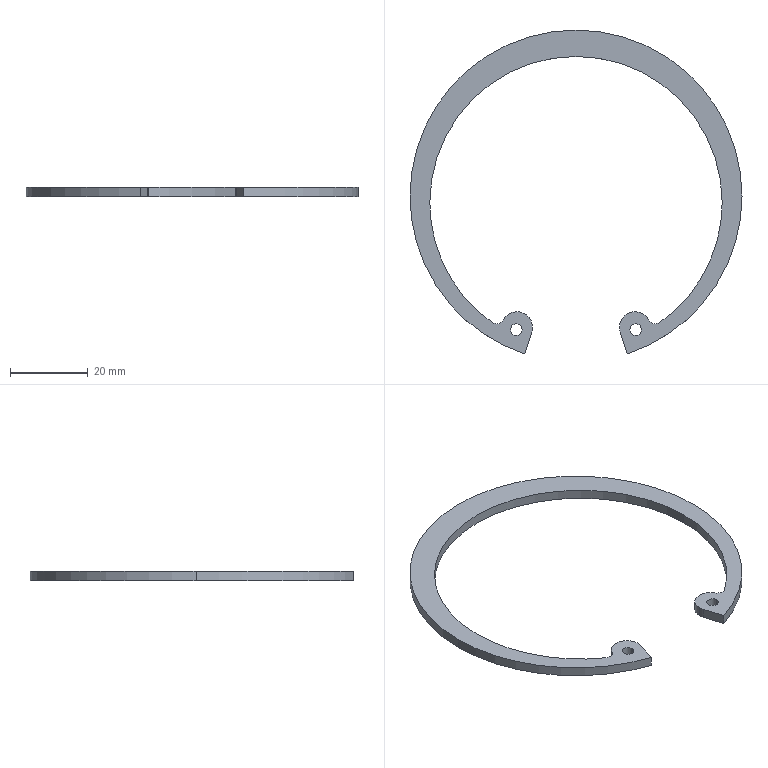Part | SolidWorks | features Extrusion 1 | 1 solid | 19 faces | box 85.5 x 83.408 x 2.5 mm | volume 3180 mm3 | cylinder 15 | plane 4 | commonest cylinder face diameters 3 x4 8 x3 75.3 x3 85.5 x3 4 x2
STEP:
#1=CARTESIAN_POINT('',(13.888,-34.416,1.25));
#2=VERTEX_POINT('',#1);
#3=CARTESIAN_POINT('',(16.888,-34.416,1.25));
#4=VERTEX_POINT('',#3);
#5=CARTESIAN_POINT('',(15.388,-34.416,1.25));
#6=DIRECTION('',(0.,0.,1.));
#7=DIRECTION('',(-1.,0.,0.));
#8=AXIS2_PLACEMENT_3D('',#5,#6,#7);
#9=CIRCLE('',#8,1.5);
#10=EDGE_CURVE('',#2,#4,#9,.T.);
#11=ORIENTED_EDGE('',*,*,#10,.T.);
#12=CARTESIAN_POINT('',(16.888,-34.416,-1.25));
#13=VERTEX_POINT('',#12);
#14=CARTESIAN_POINT('',(16.888,-34.416,1.25));
#15=DIRECTION('',(0.,0.,-1.));
#16=VECTOR('',#15,1000.);
#17=LINE('',#14,#16);
#18=EDGE_CURVE('',#4,#13,#17,.T.);
#19=ORIENTED_EDGE('',*,*,#18,.T.);
#20=CARTESIAN_POINT('',(13.888,-34.416,-1.25));
#21=VERTEX_POINT('',#20);
#22=CARTESIAN_POINT('',(15.388,-34.416,-1.25));
#23=DIRECTION('',(0.,0.,1.));
#24=DIRECTION('',(-1.,0.,0.));
#25=AXIS2_PLACEMENT_3D('',#22,#23,#24);
#26=CIRCLE('',#25,1.5);
#27=EDGE_CURVE('',#21,#13,#26,.T.);
#28=ORIENTED_EDGE('',*,*,#27,.F.);
#29=CARTESIAN_POINT('',(13.888,-34.416,1.25));
#30=DIRECTION('',(0.,0.,-1.));
#31=VECTOR('',#30,1000.);
#32=LINE('',#29,#31);
#33=EDGE_CURVE('',#2,#21,#32,.T.);
#34=ORIENTED_EDGE('',*,*,#33,.F.);
#35=EDGE_LOOP('',(#11,#19,#28,#34));
#36=FACE_OUTER_BOUND('',#35,.T.);
#37=CARTESIAN_POINT('',(15.388,-34.416,1.25));
#38=DIRECTION('',(0.,0.,-1.));
#39=DIRECTION('',(-1.,0.,0.));
#40=AXIS2_PLACEMENT_3D('',#37,#38,#39);
#41=CYLINDRICAL_SURFACE('',#40,1.5);
#42=ADVANCED_FACE('',(#36),#41,.F.);
#43=CARTESIAN_POINT('',(-16.888,-34.416,1.25));
#44=VERTEX_POINT('',#43);
#45=CARTESIAN_POINT('',(-13.888,-34.416,1.25));
#46=VERTEX_POINT('',#45);
#47=CARTESIAN_POINT('',(-15.388,-34.416,1.25));
#48=DIRECTION('',(0.,0.,1.));
#49=DIRECTION('',(1.,0.,0.));
#50=AXIS2_PLACEMENT_3D('',#47,#48,#49);
#51=CIRCLE('',#50,1.5);
#52=EDGE_CURVE('',#44,#46,#51,.T.);
#53=ORIENTED_EDGE('',*,*,#52,.T.);
#54=CARTESIAN_POINT('',(-13.888,-34.416,-1.25));
#55=VERTEX_POINT('',#54);
#56=CARTESIAN_POINT('',(-13.888,-34.416,1.25));
#57=DIRECTION('',(0.,0.,-1.));
#58=VECTOR('',#57,1000.);
#59=LINE('',#56,#58);
#60=EDGE_CURVE('',#46,#55,#59,.T.);
#61=ORIENTED_EDGE('',*,*,#60,.T.);
#62=CARTESIAN_POINT('',(-16.888,-34.416,-1.25));
#63=VERTEX_POINT('',#62);
#64=CARTESIAN_POINT('',(-15.388,-34.416,-1.25));
#65=DIRECTION('',(0.,0.,1.));
#66=DIRECTION('',(1.,0.,0.));
#67=AXIS2_PLACEMENT_3D('',#64,#65,#66);
#68=CIRCLE('',#67,1.5);
#69=EDGE_CURVE('',#63,#55,#68,.T.);
#70=ORIENTED_EDGE('',*,*,#69,.F.);
#71=CARTESIAN_POINT('',(-16.888,-34.416,1.25));
#72=DIRECTION('',(0.,0.,-1.));
#73=VECTOR('',#72,1000.);
#74=LINE('',#71,#73);
#75=EDGE_CURVE('',#44,#63,#74,.T.);
#76=ORIENTED_EDGE('',*,*,#75,.F.);
#77=EDGE_LOOP('',(#53,#61,#70,#76));
#78=FACE_OUTER_BOUND('',#77,.T.);
#79=CARTESIAN_POINT('',(-15.388,-34.416,1.25));
#80=DIRECTION('',(0.,0.,-1.));
#81=DIRECTION('',(-1.,0.,0.));
#82=AXIS2_PLACEMENT_3D('',#79,#80,#81);
#83=CYLINDRICAL_SURFACE('',#82,1.5);
#84=ADVANCED_FACE('',(#78),#83,.F.);
#85=CARTESIAN_POINT('',(42.75,0.,1.25));
#86=VERTEX_POINT('',#85);
#87=CARTESIAN_POINT('',(-42.75,0.,1.25));
#88=VERTEX_POINT('',#87);
#89=CARTESIAN_POINT('',(0.,0.,1.25));
#90=DIRECTION('',(0.,0.,1.));
#91=DIRECTION('',(1.,0.,0.));
#92=AXIS2_PLACEMENT_3D('',#89,#90,#91);
#93=CIRCLE('',#92,42.75);
#94=EDGE_CURVE('',#86,#88,#93,.T.);
#95=ORIENTED_EDGE('',*,*,#94,.F.);
#96=CARTESIAN_POINT('',(42.75,0.,-1.25));
#97=VERTEX_POINT('',#96);
#98=CARTESIAN_POINT('',(42.75,0.,1.25));
#99=DIRECTION('',(0.,0.,-1.));
#100=VECTOR('',#99,1000.);
#101=LINE('',#98,#100);
#102=EDGE_CURVE('',#86,#97,#101,.T.);
#103=ORIENTED_EDGE('',*,*,#102,.T.);
#104=CARTESIAN_POINT('',(-42.75,0.,-1.25));
#105=VERTEX_POINT('',#104);
#106=CARTESIAN_POINT('',(0.,0.,-1.25));
#107=DIRECTION('',(0.,0.,1.));
#108=DIRECTION('',(1.,0.,0.));
#109=AXIS2_PLACEMENT_3D('',#106,#107,#108);
#110=CIRCLE('',#109,42.75);
#111=EDGE_CURVE('',#97,#105,#110,.T.);
#112=ORIENTED_EDGE('',*,*,#111,.T.);
#113=CARTESIAN_POINT('',(-42.75,0.,1.25));
#114=DIRECTION('',(0.,0.,-1.));
#115=VECTOR('',#114,1000.);
#116=LINE('',#113,#115);
#117=EDGE_CURVE('',#88,#105,#116,.T.);
#118=ORIENTED_EDGE('',*,*,#117,.F.);
#119=EDGE_LOOP('',(#95,#103,#112,#118));
#120=FACE_OUTER_BOUND('',#119,.T.);
#121=CARTESIAN_POINT('',(0.,0.,1.25));
#122=DIRECTION('',(0.,0.,-1.));
#123=DIRECTION('',(-1.,0.,0.));
#124=AXIS2_PLACEMENT_3D('',#121,#122,#123);
#125=CYLINDRICAL_SURFACE('',#124,42.75);
#126=ADVANCED_FACE('',(#120),#125,.T.);
#127=CARTESIAN_POINT('',(-13.21,-40.658,1.25));
#128=VERTEX_POINT('',#127);
#129=CARTESIAN_POINT('',(0.,0.,1.25));
#130=DIRECTION('',(0.,0.,1.));
#131=DIRECTION('',(1.,0.,0.));
#132=AXIS2_PLACEMENT_3D('',#129,#130,#131);
#133=CIRCLE('',#132,42.75);
#134=EDGE_CURVE('',#88,#128,#133,.T.);
#135=ORIENTED_EDGE('',*,*,#134,.F.);
#136=ORIENTED_EDGE('',*,*,#117,.T.);
#137=CARTESIAN_POINT('',(-13.21,-40.658,-1.25));
#138=VERTEX_POINT('',#137);
#139=CARTESIAN_POINT('',(0.,0.,-1.25));
#140=DIRECTION('',(0.,0.,1.));
#141=DIRECTION('',(1.,0.,0.));
#142=AXIS2_PLACEMENT_3D('',#139,#140,#141);
#143=CIRCLE('',#142,42.75);
#144=EDGE_CURVE('',#105,#138,#143,.T.);
#145=ORIENTED_EDGE('',*,*,#144,.T.);
#146=CARTESIAN_POINT('',(-13.21,-40.658,1.25));
#147=DIRECTION('',(0.,0.,-1.));
#148=VECTOR('',#147,1000.);
#149=LINE('',#146,#148);
#150=EDGE_CURVE('',#128,#138,#149,.T.);
#151=ORIENTED_EDGE('',*,*,#150,.F.);
#152=EDGE_LOOP('',(#135,#136,#145,#151));
#153=FACE_OUTER_BOUND('',#152,.T.);
#154=CARTESIAN_POINT('',(0.,0.,1.25));
#155=DIRECTION('',(0.,0.,-1.));
#156=DIRECTION('',(-1.,0.,0.));
#157=AXIS2_PLACEMENT_3D('',#154,#155,#156);
#158=CYLINDRICAL_SURFACE('',#157,42.75);
#159=ADVANCED_FACE('',(#153),#158,.T.);
#160=CARTESIAN_POINT('',(11.186,-33.795,1.25));
#161=VERTEX_POINT('',#160);
#162=CARTESIAN_POINT('',(11.382,-35.031,1.25));
#163=VERTEX_POINT('',#162);
#164=CARTESIAN_POINT('',(15.186,-33.795,1.25));
#165=DIRECTION('',(0.,0.,1.));
#166=DIRECTION('',(-1.,0.,0.));
#167=AXIS2_PLACEMENT_3D('',#164,#165,#166);
#168=CIRCLE('',#167,4.);
#169=EDGE_CURVE('',#161,#163,#168,.T.);
#170=ORIENTED_EDGE('',*,*,#169,.F.);
#171=CARTESIAN_POINT('',(11.186,-33.795,-1.25));
#172=VERTEX_POINT('',#171);
#173=CARTESIAN_POINT('',(11.186,-33.795,1.25));
#174=DIRECTION('',(0.,0.,-1.));
#175=VECTOR('',#174,1000.);
#176=LINE('',#173,#175);
#177=EDGE_CURVE('',#161,#172,#176,.T.);
#178=ORIENTED_EDGE('',*,*,#177,.T.);
#179=CARTESIAN_POINT('',(11.382,-35.031,-1.25));
#180=VERTEX_POINT('',#179);
#181=CARTESIAN_POINT('',(15.186,-33.795,-1.25));
#182=DIRECTION('',(0.,0.,1.));
#183=DIRECTION('',(-1.,0.,0.));
#184=AXIS2_PLACEMENT_3D('',#181,#182,#183);
#185=CIRCLE('',#184,4.);
#186=EDGE_CURVE('',#172,#180,#185,.T.);
#187=ORIENTED_EDGE('',*,*,#186,.T.);
#188=CARTESIAN_POINT('',(11.382,-35.031,1.25));
#189=DIRECTION('',(0.,0.,-1.));
#190=VECTOR('',#189,1000.);
#191=LINE('',#188,#190);
#192=EDGE_CURVE('',#163,#180,#191,.T.);
#193=ORIENTED_EDGE('',*,*,#192,.F.);
#194=EDGE_LOOP('',(#170,#178,#187,#193));
#195=FACE_OUTER_BOUND('',#194,.T.);
#196=CARTESIAN_POINT('',(15.186,-33.795,1.25));
#197=DIRECTION('',(0.,0.,-1.));
#198=DIRECTION('',(-1.,0.,0.));
#199=AXIS2_PLACEMENT_3D('',#196,#197,#198);
#200=CYLINDRICAL_SURFACE('',#199,4.);
#201=ADVANCED_FACE('',(#195),#200,.T.);
#202=CARTESIAN_POINT('',(37.65,-1.7,1.25));
#203=VERTEX_POINT('',#202);
#204=CARTESIAN_POINT('',(21.592,-32.543,1.25));
#205=VERTEX_POINT('',#204);
#206=CARTESIAN_POINT('',(0.,-1.7,1.25));
#207=DIRECTION('',(0.,0.,-1.));
#208=DIRECTION('',(1.,0.,0.));
#209=AXIS2_PLACEMENT_3D('',#206,#207,#208);
#210=CIRCLE('',#209,37.65);
#211=EDGE_CURVE('',#203,#205,#210,.T.);
#212=ORIENTED_EDGE('',*,*,#211,.F.);
#213=CARTESIAN_POINT('',(37.65,-1.7,-1.25));
#214=VERTEX_POINT('',#213);
#215=CARTESIAN_POINT('',(37.65,-1.7,1.25));
#216=DIRECTION('',(0.,0.,-1.));
#217=VECTOR('',#216,1000.);
#218=LINE('',#215,#217);
#219=EDGE_CURVE('',#203,#214,#218,.T.);
#220=ORIENTED_EDGE('',*,*,#219,.T.);
#221=CARTESIAN_POINT('',(21.592,-32.543,-1.25));
#222=VERTEX_POINT('',#221);
#223=CARTESIAN_POINT('',(0.,-1.7,-1.25));
#224=DIRECTION('',(0.,0.,-1.));
#225=DIRECTION('',(1.,0.,0.));
#226=AXIS2_PLACEMENT_3D('',#223,#224,#225);
#227=CIRCLE('',#226,37.65);
#228=EDGE_CURVE('',#214,#222,#227,.T.);
#229=ORIENTED_EDGE('',*,*,#228,.T.);
#230=CARTESIAN_POINT('',(21.592,-32.543,1.25));
#231=DIRECTION('',(0.,0.,-1.));
#232=VECTOR('',#231,1000.);
#233=LINE('',#230,#232);
#234=EDGE_CURVE('',#205,#222,#233,.T.);
#235=ORIENTED_EDGE('',*,*,#234,.F.);
#236=EDGE_LOOP('',(#212,#220,#229,#235));
#237=FACE_OUTER_BOUND('',#236,.T.);
#238=CARTESIAN_POINT('',(0.,-1.7,1.25));
#239=DIRECTION('',(0.,0.,-1.));
#240=DIRECTION('',(-1.,0.,0.));
#241=AXIS2_PLACEMENT_3D('',#238,#239,#240);
#242=CYLINDRICAL_SURFACE('',#241,37.65);
#243=ADVANCED_FACE('',(#237),#242,.F.);
#244=ORIENTED_EDGE('',*,*,#219,.F.);
#245=CARTESIAN_POINT('',(-37.65,-1.7,1.25));
#246=VERTEX_POINT('',#245);
#247=CARTESIAN_POINT('',(0.,-1.7,1.25));
#248=DIRECTION('',(0.,0.,-1.));
#249=DIRECTION('',(1.,0.,0.));
#250=AXIS2_PLACEMENT_3D('',#247,#248,#249);
#251=CIRCLE('',#250,37.65);
#252=EDGE_CURVE('',#246,#203,#251,.T.);
#253=ORIENTED_EDGE('',*,*,#252,.F.);
#254=CARTESIAN_POINT('',(-37.65,-1.7,-1.25));
#255=VERTEX_POINT('',#254);
#256=CARTESIAN_POINT('',(-37.65,-1.7,1.25));
#257=DIRECTION('',(0.,0.,-1.));
#258=VECTOR('',#257,1000.);
#259=LINE('',#256,#258);
#260=EDGE_CURVE('',#246,#255,#259,.T.);
#261=ORIENTED_EDGE('',*,*,#260,.T.);
#262=CARTESIAN_POINT('',(0.,-1.7,-1.25));
#263=DIRECTION('',(0.,0.,-1.));
#264=DIRECTION('',(1.,0.,0.));
#265=AXIS2_PLACEMENT_3D('',#262,#263,#264);
#266=CIRCLE('',#265,37.65);
#267=EDGE_CURVE('',#255,#214,#266,.T.);
#268=ORIENTED_EDGE('',*,*,#267,.T.);
#269=EDGE_LOOP('',(#244,#253,#261,#268));
#270=FACE_OUTER_BOUND('',#269,.T.);
#271=CARTESIAN_POINT('',(0.,-1.7,1.25));
#272=DIRECTION('',(0.,0.,-1.));
#273=DIRECTION('',(-1.,0.,0.));
#274=AXIS2_PLACEMENT_3D('',#271,#272,#273);
#275=CYLINDRICAL_SURFACE('',#274,37.65);
#276=ADVANCED_FACE('',(#270),#275,.F.);
#277=ORIENTED_EDGE('',*,*,#52,.F.);
#278=CARTESIAN_POINT('',(-15.388,-34.416,1.25));
#279=DIRECTION('',(0.,0.,1.));
#280=DIRECTION('',(1.,0.,0.));
#281=AXIS2_PLACEMENT_3D('',#278,#279,#280);
#282=CIRCLE('',#281,1.5);
#283=EDGE_CURVE('',#46,#44,#282,.T.);
#284=ORIENTED_EDGE('',*,*,#283,.F.);
#285=EDGE_LOOP('',(#277,#284));
#286=FACE_BOUND('',#285,.T.);
#287=CARTESIAN_POINT('',(-11.382,-35.031,1.25));
#288=VERTEX_POINT('',#287);
#289=CARTESIAN_POINT('',(-18.692,-31.868,1.25));
#290=VERTEX_POINT('',#289);
#291=CARTESIAN_POINT('',(-15.186,-33.795,1.25));
#292=DIRECTION('',(0.,0.,1.));
#293=DIRECTION('',(1.,0.,0.));
#294=AXIS2_PLACEMENT_3D('',#291,#292,#293);
#295=CIRCLE('',#294,4.);
#296=EDGE_CURVE('',#288,#290,#295,.T.);
#297=ORIENTED_EDGE('',*,*,#296,.T.);
#298=CARTESIAN_POINT('',(-21.592,-32.543,1.25));
#299=VERTEX_POINT('',#298);
#300=CARTESIAN_POINT('',(-20.445,-30.905,1.25));
#301=DIRECTION('',(0.,0.,-1.));
#302=DIRECTION('',(-1.,0.,0.));
#303=AXIS2_PLACEMENT_3D('',#300,#301,#302);
#304=CIRCLE('',#303,2.);
#305=EDGE_CURVE('',#290,#299,#304,.T.);
#306=ORIENTED_EDGE('',*,*,#305,.T.);
#307=CARTESIAN_POINT('',(0.,-1.7,1.25));
#308=DIRECTION('',(0.,0.,-1.));
#309=DIRECTION('',(1.,0.,0.));
#310=AXIS2_PLACEMENT_3D('',#307,#308,#309);
#311=CIRCLE('',#310,37.65);
#312=EDGE_CURVE('',#299,#246,#311,.T.);
#313=ORIENTED_EDGE('',*,*,#312,.T.);
#314=ORIENTED_EDGE('',*,*,#252,.T.);
#315=ORIENTED_EDGE('',*,*,#211,.T.);
#316=CARTESIAN_POINT('',(18.692,-31.868,1.25));
#317=VERTEX_POINT('',#316);
#318=CARTESIAN_POINT('',(20.445,-30.905,1.25));
#319=DIRECTION('',(0.,0.,-1.));
#320=DIRECTION('',(1.,0.,0.));
#321=AXIS2_PLACEMENT_3D('',#318,#319,#320);
#322=CIRCLE('',#321,2.);
#323=EDGE_CURVE('',#205,#317,#322,.T.);
#324=ORIENTED_EDGE('',*,*,#323,.T.);
#325=CARTESIAN_POINT('',(15.186,-33.795,1.25));
#326=DIRECTION('',(0.,0.,1.));
#327=DIRECTION('',(-1.,0.,0.));
#328=AXIS2_PLACEMENT_3D('',#325,#326,#327);
#329=CIRCLE('',#328,4.);
#330=EDGE_CURVE('',#317,#161,#329,.T.);
#331=ORIENTED_EDGE('',*,*,#330,.T.);
#332=ORIENTED_EDGE('',*,*,#169,.T.);
#333=CARTESIAN_POINT('',(13.21,-40.658,1.25));
#334=VERTEX_POINT('',#333);
#335=CARTESIAN_POINT('',(11.382,-35.031,1.25));
#336=DIRECTION('',(0.309,-0.9511,0.));
#337=VECTOR('',#336,1000.);
#338=LINE('',#335,#337);
#339=EDGE_CURVE('',#163,#334,#338,.T.);
#340=ORIENTED_EDGE('',*,*,#339,.T.);
#341=CARTESIAN_POINT('',(0.,0.,1.25));
#342=DIRECTION('',(0.,0.,1.));
#343=DIRECTION('',(1.,0.,0.));
#344=AXIS2_PLACEMENT_3D('',#341,#342,#343);
#345=CIRCLE('',#344,42.75);
#346=EDGE_CURVE('',#334,#86,#345,.T.);
#347=ORIENTED_EDGE('',*,*,#346,.T.);
#348=ORIENTED_EDGE('',*,*,#94,.T.);
#349=ORIENTED_EDGE('',*,*,#134,.T.);
#350=CARTESIAN_POINT('',(-11.382,-35.031,1.25));
#351=DIRECTION('',(0.309,0.9511,0.));
#352=VECTOR('',#351,1000.);
#353=LINE('',#350,#352);
#354=EDGE_CURVE('',#128,#288,#353,.T.);
#355=ORIENTED_EDGE('',*,*,#354,.T.);
#356=EDGE_LOOP('',(#297,#306,#313,#314,#315,#324,#331,#332,#340,#347,#348,#349,#355));
#357=FACE_OUTER_BOUND('',#356,.T.);
#358=ORIENTED_EDGE('',*,*,#10,.F.);
#359=CARTESIAN_POINT('',(15.388,-34.416,1.25));
#360=DIRECTION('',(0.,0.,1.));
#361=DIRECTION('',(-1.,0.,0.));
#362=AXIS2_PLACEMENT_3D('',#359,#360,#361);
#363=CIRCLE('',#362,1.5);
#364=EDGE_CURVE('',#4,#2,#363,.T.);
#365=ORIENTED_EDGE('',*,*,#364,.F.);
#366=EDGE_LOOP('',(#358,#365));
#367=FACE_BOUND('',#366,.T.);
#368=CARTESIAN_POINT('',(-15.186,-33.795,1.25));
#369=DIRECTION('',(0.,0.,1.));
#370=DIRECTION('',(1.,0.,0.));
#371=AXIS2_PLACEMENT_3D('',#368,#369,#370);
#372=PLANE('',#371);
#373=ADVANCED_FACE('',(#286,#357,#367),#372,.T.);
#374=CARTESIAN_POINT('',(-11.382,-35.031,-1.25));
#375=VERTEX_POINT('',#374);
#376=CARTESIAN_POINT('',(-11.382,-35.031,1.25));
#377=DIRECTION('',(0.,0.,-1.));
#378=VECTOR('',#377,1000.);
#379=LINE('',#376,#378);
#380=EDGE_CURVE('',#288,#375,#379,.T.);
#381=ORIENTED_EDGE('',*,*,#380,.T.);
#382=CARTESIAN_POINT('',(-18.692,-31.868,-1.25));
#383=VERTEX_POINT('',#382);
#384=CARTESIAN_POINT('',(-15.186,-33.795,-1.25));
#385=DIRECTION('',(0.,0.,1.));
#386=DIRECTION('',(1.,0.,0.));
#387=AXIS2_PLACEMENT_3D('',#384,#385,#386);
#388=CIRCLE('',#387,4.);
#389=EDGE_CURVE('',#375,#383,#388,.T.);
#390=ORIENTED_EDGE('',*,*,#389,.T.);
#391=CARTESIAN_POINT('',(-18.692,-31.868,1.25));
#392=DIRECTION('',(0.,0.,-1.));
#393=VECTOR('',#392,1000.);
#394=LINE('',#391,#393);
#395=EDGE_CURVE('',#290,#383,#394,.T.);
#396=ORIENTED_EDGE('',*,*,#395,.F.);
#397=ORIENTED_EDGE('',*,*,#296,.F.);
#398=EDGE_LOOP('',(#381,#390,#396,#397));
#399=FACE_OUTER_BOUND('',#398,.T.);
#400=CARTESIAN_POINT('',(-15.186,-33.795,1.25));
#401=DIRECTION('',(0.,0.,-1.));
#402=DIRECTION('',(-1.,0.,0.));
#403=AXIS2_PLACEMENT_3D('',#400,#401,#402);
#404=CYLINDRICAL_SURFACE('',#403,4.);
#405=ADVANCED_FACE('',(#399),#404,.T.);
#406=ORIENTED_EDGE('',*,*,#395,.T.);
#407=CARTESIAN_POINT('',(-21.592,-32.543,-1.25));
#408=VERTEX_POINT('',#407);
#409=CARTESIAN_POINT('',(-20.445,-30.905,-1.25));
#410=DIRECTION('',(0.,0.,-1.));
#411=DIRECTION('',(-1.,0.,0.));
#412=AXIS2_PLACEMENT_3D('',#409,#410,#411);
#413=CIRCLE('',#412,2.);
#414=EDGE_CURVE('',#383,#408,#413,.T.);
#415=ORIENTED_EDGE('',*,*,#414,.T.);
#416=CARTESIAN_POINT('',(-21.592,-32.543,1.25));
#417=DIRECTION('',(0.,0.,-1.));
#418=VECTOR('',#417,1000.);
#419=LINE('',#416,#418);
#420=EDGE_CURVE('',#299,#408,#419,.T.);
#421=ORIENTED_EDGE('',*,*,#420,.F.);
#422=ORIENTED_EDGE('',*,*,#305,.F.);
#423=EDGE_LOOP('',(#406,#415,#421,#422));
#424=FACE_OUTER_BOUND('',#423,.T.);
#425=CARTESIAN_POINT('',(-20.445,-30.905,1.25));
#426=DIRECTION('',(0.,0.,-1.));
#427=DIRECTION('',(-1.,0.,0.));
#428=AXIS2_PLACEMENT_3D('',#425,#426,#427);
#429=CYLINDRICAL_SURFACE('',#428,2.);
#430=ADVANCED_FACE('',(#424),#429,.F.);
#431=ORIENTED_EDGE('',*,*,#260,.F.);
#432=ORIENTED_EDGE('',*,*,#312,.F.);
#433=ORIENTED_EDGE('',*,*,#420,.T.);
#434=CARTESIAN_POINT('',(0.,-1.7,-1.25));
#435=DIRECTION('',(0.,0.,-1.));
#436=DIRECTION('',(1.,0.,0.));
#437=AXIS2_PLACEMENT_3D('',#434,#435,#436);
#438=CIRCLE('',#437,37.65);
#439=EDGE_CURVE('',#408,#255,#438,.T.);
#440=ORIENTED_EDGE('',*,*,#439,.T.);
#441=EDGE_LOOP('',(#431,#432,#433,#440));
#442=FACE_OUTER_BOUND('',#441,.T.);
#443=CARTESIAN_POINT('',(0.,-1.7,1.25));
#444=DIRECTION('',(0.,0.,-1.));
#445=DIRECTION('',(-1.,0.,0.));
#446=AXIS2_PLACEMENT_3D('',#443,#444,#445);
#447=CYLINDRICAL_SURFACE('',#446,37.65);
#448=ADVANCED_FACE('',(#442),#447,.F.);
#449=ORIENTED_EDGE('',*,*,#234,.T.);
#450=CARTESIAN_POINT('',(18.692,-31.868,-1.25));
#451=VERTEX_POINT('',#450);
#452=CARTESIAN_POINT('',(20.445,-30.905,-1.25));
#453=DIRECTION('',(0.,0.,-1.));
#454=DIRECTION('',(1.,0.,0.));
#455=AXIS2_PLACEMENT_3D('',#452,#453,#454);
#456=CIRCLE('',#455,2.);
#457=EDGE_CURVE('',#222,#451,#456,.T.);
#458=ORIENTED_EDGE('',*,*,#457,.T.);
#459=CARTESIAN_POINT('',(18.692,-31.868,1.25));
#460=DIRECTION('',(0.,0.,-1.));
#461=VECTOR('',#460,1000.);
#462=LINE('',#459,#461);
#463=EDGE_CURVE('',#317,#451,#462,.T.);
#464=ORIENTED_EDGE('',*,*,#463,.F.);
#465=ORIENTED_EDGE('',*,*,#323,.F.);
#466=EDGE_LOOP('',(#449,#458,#464,#465));
#467=FACE_OUTER_BOUND('',#466,.T.);
#468=CARTESIAN_POINT('',(20.445,-30.905,1.25));
#469=DIRECTION('',(0.,0.,-1.));
#470=DIRECTION('',(-1.,0.,0.));
#471=AXIS2_PLACEMENT_3D('',#468,#469,#470);
#472=CYLINDRICAL_SURFACE('',#471,2.);
#473=ADVANCED_FACE('',(#467),#472,.F.);
#474=ORIENTED_EDGE('',*,*,#177,.F.);
#475=ORIENTED_EDGE('',*,*,#330,.F.);
#476=ORIENTED_EDGE('',*,*,#463,.T.);
#477=CARTESIAN_POINT('',(15.186,-33.795,-1.25));
#478=DIRECTION('',(0.,0.,1.));
#479=DIRECTION('',(-1.,0.,0.));
#480=AXIS2_PLACEMENT_3D('',#477,#478,#479);
#481=CIRCLE('',#480,4.);
#482=EDGE_CURVE('',#451,#172,#481,.T.);
#483=ORIENTED_EDGE('',*,*,#482,.T.);
#484=EDGE_LOOP('',(#474,#475,#476,#483));
#485=FACE_OUTER_BOUND('',#484,.T.);
#486=CARTESIAN_POINT('',(15.186,-33.795,1.25));
#487=DIRECTION('',(0.,0.,-1.));
#488=DIRECTION('',(-1.,0.,0.));
#489=AXIS2_PLACEMENT_3D('',#486,#487,#488);
#490=CYLINDRICAL_SURFACE('',#489,4.);
#491=ADVANCED_FACE('',(#485),#490,.T.);
#492=ORIENTED_EDGE('',*,*,#192,.T.);
#493=CARTESIAN_POINT('',(13.21,-40.658,-1.25));
#494=VERTEX_POINT('',#493);
#495=CARTESIAN_POINT('',(11.382,-35.031,-1.25));
#496=DIRECTION('',(0.309,-0.9511,0.));
#497=VECTOR('',#496,1000.);
#498=LINE('',#495,#497);
#499=EDGE_CURVE('',#180,#494,#498,.T.);
#500=ORIENTED_EDGE('',*,*,#499,.T.);
#501=CARTESIAN_POINT('',(13.21,-40.658,1.25));
#502=DIRECTION('',(0.,0.,-1.));
#503=VECTOR('',#502,1000.);
#504=LINE('',#501,#503);
#505=EDGE_CURVE('',#334,#494,#504,.T.);
#506=ORIENTED_EDGE('',*,*,#505,.F.);
#507=ORIENTED_EDGE('',*,*,#339,.F.);
#508=EDGE_LOOP('',(#492,#500,#506,#507));
#509=FACE_OUTER_BOUND('',#508,.T.);
#510=CARTESIAN_POINT('',(11.382,-35.031,1.25));
#511=DIRECTION('',(0.9511,0.309,0.));
#512=DIRECTION('',(-0.309,0.9511,0.));
#513=AXIS2_PLACEMENT_3D('',#510,#511,#512);
#514=PLANE('',#513);
#515=ADVANCED_FACE('',(#509),#514,.F.);
#516=ORIENTED_EDGE('',*,*,#102,.F.);
#517=ORIENTED_EDGE('',*,*,#346,.F.);
#518=ORIENTED_EDGE('',*,*,#505,.T.);
#519=CARTESIAN_POINT('',(0.,0.,-1.25));
#520=DIRECTION('',(0.,0.,1.));
#521=DIRECTION('',(1.,0.,0.));
#522=AXIS2_PLACEMENT_3D('',#519,#520,#521);
#523=CIRCLE('',#522,42.75);
#524=EDGE_CURVE('',#494,#97,#523,.T.);
#525=ORIENTED_EDGE('',*,*,#524,.T.);
#526=EDGE_LOOP('',(#516,#517,#518,#525));
#527=FACE_OUTER_BOUND('',#526,.T.);
#528=CARTESIAN_POINT('',(0.,0.,1.25));
#529=DIRECTION('',(0.,0.,-1.));
#530=DIRECTION('',(-1.,0.,0.));
#531=AXIS2_PLACEMENT_3D('',#528,#529,#530);
#532=CYLINDRICAL_SURFACE('',#531,42.75);
#533=ADVANCED_FACE('',(#527),#532,.T.);
#534=ORIENTED_EDGE('',*,*,#150,.T.);
#535=CARTESIAN_POINT('',(-11.382,-35.031,-1.25));
#536=DIRECTION('',(0.309,0.9511,0.));
#537=VECTOR('',#536,1000.);
#538=LINE('',#535,#537);
#539=EDGE_CURVE('',#138,#375,#538,.T.);
#540=ORIENTED_EDGE('',*,*,#539,.T.);
#541=ORIENTED_EDGE('',*,*,#380,.F.);
#542=ORIENTED_EDGE('',*,*,#354,.F.);
#543=EDGE_LOOP('',(#534,#540,#541,#542));
#544=FACE_OUTER_BOUND('',#543,.T.);
#545=CARTESIAN_POINT('',(-11.382,-35.031,1.25));
#546=DIRECTION('',(-0.9511,0.309,0.));
#547=DIRECTION('',(-0.309,-0.9511,0.));
#548=AXIS2_PLACEMENT_3D('',#545,#546,#547);
#549=PLANE('',#548);
#550=ADVANCED_FACE('',(#544),#549,.F.);
#551=ORIENTED_EDGE('',*,*,#60,.F.);
#552=ORIENTED_EDGE('',*,*,#283,.T.);
#553=ORIENTED_EDGE('',*,*,#75,.T.);
#554=CARTESIAN_POINT('',(-15.388,-34.416,-1.25));
#555=DIRECTION('',(0.,0.,1.));
#556=DIRECTION('',(1.,0.,0.));
#557=AXIS2_PLACEMENT_3D('',#554,#555,#556);
#558=CIRCLE('',#557,1.5);
#559=EDGE_CURVE('',#55,#63,#558,.T.);
#560=ORIENTED_EDGE('',*,*,#559,.F.);
#561=EDGE_LOOP('',(#551,#552,#553,#560));
#562=FACE_OUTER_BOUND('',#561,.T.);
#563=CARTESIAN_POINT('',(-15.388,-34.416,1.25));
#564=DIRECTION('',(0.,0.,-1.));
#565=DIRECTION('',(-1.,0.,0.));
#566=AXIS2_PLACEMENT_3D('',#563,#564,#565);
#567=CYLINDRICAL_SURFACE('',#566,1.5);
#568=ADVANCED_FACE('',(#562),#567,.F.);
#569=ORIENTED_EDGE('',*,*,#18,.F.);
#570=ORIENTED_EDGE('',*,*,#364,.T.);
#571=ORIENTED_EDGE('',*,*,#33,.T.);
#572=CARTESIAN_POINT('',(15.388,-34.416,-1.25));
#573=DIRECTION('',(0.,0.,1.));
#574=DIRECTION('',(-1.,0.,0.));
#575=AXIS2_PLACEMENT_3D('',#572,#573,#574);
#576=CIRCLE('',#575,1.5);
#577=EDGE_CURVE('',#13,#21,#576,.T.);
#578=ORIENTED_EDGE('',*,*,#577,.F.);
#579=EDGE_LOOP('',(#569,#570,#571,#578));
#580=FACE_OUTER_BOUND('',#579,.T.);
#581=CARTESIAN_POINT('',(15.388,-34.416,1.25));
#582=DIRECTION('',(0.,0.,-1.));
#583=DIRECTION('',(-1.,0.,0.));
#584=AXIS2_PLACEMENT_3D('',#581,#582,#583);
#585=CYLINDRICAL_SURFACE('',#584,1.5);
#586=ADVANCED_FACE('',(#580),#585,.F.);
#587=ORIENTED_EDGE('',*,*,#27,.T.);
#588=ORIENTED_EDGE('',*,*,#577,.T.);
#589=EDGE_LOOP('',(#587,#588));
#590=FACE_BOUND('',#589,.T.);
#591=ORIENTED_EDGE('',*,*,#69,.T.);
#592=ORIENTED_EDGE('',*,*,#559,.T.);
#593=EDGE_LOOP('',(#591,#592));
#594=FACE_BOUND('',#593,.T.);
#595=ORIENTED_EDGE('',*,*,#389,.F.);
#596=ORIENTED_EDGE('',*,*,#539,.F.);
#597=ORIENTED_EDGE('',*,*,#144,.F.);
#598=ORIENTED_EDGE('',*,*,#111,.F.);
#599=ORIENTED_EDGE('',*,*,#524,.F.);
#600=ORIENTED_EDGE('',*,*,#499,.F.);
#601=ORIENTED_EDGE('',*,*,#186,.F.);
#602=ORIENTED_EDGE('',*,*,#482,.F.);
#603=ORIENTED_EDGE('',*,*,#457,.F.);
#604=ORIENTED_EDGE('',*,*,#228,.F.);
#605=ORIENTED_EDGE('',*,*,#267,.F.);
#606=ORIENTED_EDGE('',*,*,#439,.F.);
#607=ORIENTED_EDGE('',*,*,#414,.F.);
#608=EDGE_LOOP('',(#595,#596,#597,#598,#599,#600,#601,#602,#603,#604,#605,#606,#607));
#609=FACE_OUTER_BOUND('',#608,.T.);
#610=CARTESIAN_POINT('',(-15.186,-33.795,-1.25));
#611=DIRECTION('',(0.,0.,1.));
#612=DIRECTION('',(1.,0.,0.));
#613=AXIS2_PLACEMENT_3D('',#610,#611,#612);
#614=PLANE('',#613);
#615=ADVANCED_FACE('',(#590,#594,#609),#614,.F.);
#616=CLOSED_SHELL('',(#42,#84,#126,#159,#201,#243,#276,#373,#405,#430,#448,#473,#491,#515,#533,#550,#568,#586,#615));
#617=MANIFOLD_SOLID_BREP('',#616);
#618=CARTESIAN_POINT('',(0.,0.,0.));
#619=DIRECTION('',(0.,0.,1.));
#620=DIRECTION('',(1.,0.,0.));
#621=AXIS2_PLACEMENT_3D('',#618,#619,#620);
#622=(LENGTH_UNIT()NAMED_UNIT(*)SI_UNIT(.MILLI.,.METRE.));
#623=UNCERTAINTY_MEASURE_WITH_UNIT(LENGTH_MEASURE(0.00001),#622,'','');
#624=(NAMED_UNIT(*)PLANE_ANGLE_UNIT()SI_UNIT($,.RADIAN.));
#625=(NAMED_UNIT(*)SI_UNIT($,.STERADIAN.)SOLID_ANGLE_UNIT());
#626=(GEOMETRIC_REPRESENTATION_CONTEXT(3)GLOBAL_UNCERTAINTY_ASSIGNED_CONTEXT((#623))GLOBAL_UNIT_ASSIGNED_CONTEXT((#622,#624,#625))REPRESENTATION_CONTEXT('',''));
#627=ADVANCED_BREP_SHAPE_REPRESENTATION('',(#617,#621),#626);